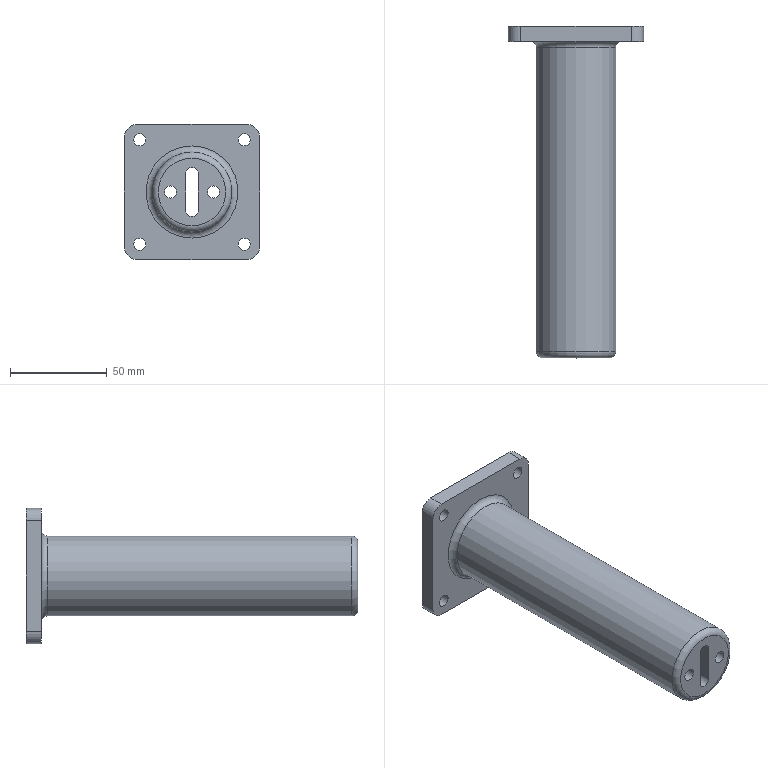Part | NX | features MG0330 trunion parts 24(stanchion group) 2 | 1 solid | 32 faces | box 69.85 x 171.45 x 69.85 mm | volume 105994 mm3 | cylinder 15 | plane 11 | torus 4 | cone 2 | commonest cylinder face diameters 6.35 x6 12.7 x4 6.401 x2 34.925 x2 41.275 x1
STEP:
#1=CARTESIAN_POINT('',(0.,285.75,17.971));
#2=VERTEX_POINT('',#1);
#3=CARTESIAN_POINT('',(0.,285.75,0.));
#4=DIRECTION('',(0.,1.,0.));
#5=DIRECTION('',(0.,0.,1.));
#6=AXIS2_PLACEMENT_3D('',#3,#4,#5);
#7=CIRCLE('',#6,17.971);
#8=EDGE_CURVE('',#2,#2,#7,.F.);
#9=ORIENTED_EDGE('',*,*,#8,.T.);
#10=EDGE_LOOP('',(#9));
#11=FACE_BOUND('',#10,.T.);
#12=CARTESIAN_POINT('',(-26.988,285.75,-23.812));
#13=VERTEX_POINT('',#12);
#14=CARTESIAN_POINT('',(-26.988,285.75,-26.988));
#15=DIRECTION('',(0.,1.,0.));
#16=DIRECTION('',(0.,0.,1.));
#17=AXIS2_PLACEMENT_3D('',#14,#15,#16);
#18=CIRCLE('',#17,3.175);
#19=EDGE_CURVE('',#13,#13,#18,.T.);
#20=ORIENTED_EDGE('',*,*,#19,.F.);
#21=EDGE_LOOP('',(#20));
#22=FACE_BOUND('',#21,.T.);
#23=CARTESIAN_POINT('',(26.988,285.75,-23.812));
#24=VERTEX_POINT('',#23);
#25=CARTESIAN_POINT('',(26.988,285.75,-26.988));
#26=DIRECTION('',(0.,1.,0.));
#27=DIRECTION('',(0.,0.,1.));
#28=AXIS2_PLACEMENT_3D('',#25,#26,#27);
#29=CIRCLE('',#28,3.175);
#30=EDGE_CURVE('',#24,#24,#29,.T.);
#31=ORIENTED_EDGE('',*,*,#30,.F.);
#32=EDGE_LOOP('',(#31));
#33=FACE_BOUND('',#32,.T.);
#34=CARTESIAN_POINT('',(26.988,285.75,30.163));
#35=VERTEX_POINT('',#34);
#36=CARTESIAN_POINT('',(26.988,285.75,26.988));
#37=DIRECTION('',(0.,1.,0.));
#38=DIRECTION('',(0.,0.,1.));
#39=AXIS2_PLACEMENT_3D('',#36,#37,#38);
#40=CIRCLE('',#39,3.175);
#41=EDGE_CURVE('',#35,#35,#40,.T.);
#42=ORIENTED_EDGE('',*,*,#41,.F.);
#43=EDGE_LOOP('',(#42));
#44=FACE_BOUND('',#43,.T.);
#45=CARTESIAN_POINT('',(-26.988,285.75,30.163));
#46=VERTEX_POINT('',#45);
#47=CARTESIAN_POINT('',(-26.988,285.75,26.988));
#48=DIRECTION('',(0.,1.,0.));
#49=DIRECTION('',(0.,0.,1.));
#50=AXIS2_PLACEMENT_3D('',#47,#48,#49);
#51=CIRCLE('',#50,3.175);
#52=EDGE_CURVE('',#46,#46,#51,.T.);
#53=ORIENTED_EDGE('',*,*,#52,.F.);
#54=EDGE_LOOP('',(#53));
#55=FACE_BOUND('',#54,.T.);
#56=CARTESIAN_POINT('',(28.575,285.75,-34.925));
#57=VERTEX_POINT('',#56);
#58=CARTESIAN_POINT('',(-28.575,285.75,-34.925));
#59=VERTEX_POINT('',#58);
#60=CARTESIAN_POINT('',(34.925,285.75,-34.925));
#61=DIRECTION('',(-1.,0.,0.));
#62=VECTOR('',#61,1000.);
#63=LINE('',#60,#62);
#64=EDGE_CURVE('',#57,#59,#63,.T.);
#65=ORIENTED_EDGE('',*,*,#64,.T.);
#66=CARTESIAN_POINT('',(-34.925,285.75,-28.575));
#67=VERTEX_POINT('',#66);
#68=CARTESIAN_POINT('',(-28.575,285.75,-28.575));
#69=DIRECTION('',(0.,1.,0.));
#70=DIRECTION('',(0.,0.,1.));
#71=AXIS2_PLACEMENT_3D('',#68,#69,#70);
#72=CIRCLE('',#71,6.35);
#73=EDGE_CURVE('',#59,#67,#72,.T.);
#74=ORIENTED_EDGE('',*,*,#73,.T.);
#75=CARTESIAN_POINT('',(-34.925,285.75,28.575));
#76=VERTEX_POINT('',#75);
#77=CARTESIAN_POINT('',(-34.925,285.75,-34.925));
#78=DIRECTION('',(0.,0.,1.));
#79=VECTOR('',#78,1000.);
#80=LINE('',#77,#79);
#81=EDGE_CURVE('',#67,#76,#80,.T.);
#82=ORIENTED_EDGE('',*,*,#81,.T.);
#83=CARTESIAN_POINT('',(-28.575,285.75,34.925));
#84=VERTEX_POINT('',#83);
#85=CARTESIAN_POINT('',(-28.575,285.75,28.575));
#86=DIRECTION('',(0.,1.,0.));
#87=DIRECTION('',(0.,0.,1.));
#88=AXIS2_PLACEMENT_3D('',#85,#86,#87);
#89=CIRCLE('',#88,6.35);
#90=EDGE_CURVE('',#76,#84,#89,.T.);
#91=ORIENTED_EDGE('',*,*,#90,.T.);
#92=CARTESIAN_POINT('',(28.575,285.75,34.925));
#93=VERTEX_POINT('',#92);
#94=CARTESIAN_POINT('',(34.925,285.75,34.925));
#95=DIRECTION('',(1.,0.,0.));
#96=VECTOR('',#95,1000.);
#97=LINE('',#94,#96);
#98=EDGE_CURVE('',#84,#93,#97,.T.);
#99=ORIENTED_EDGE('',*,*,#98,.T.);
#100=CARTESIAN_POINT('',(34.925,285.75,28.575));
#101=VERTEX_POINT('',#100);
#102=CARTESIAN_POINT('',(28.575,285.75,28.575));
#103=DIRECTION('',(0.,1.,0.));
#104=DIRECTION('',(0.,0.,1.));
#105=AXIS2_PLACEMENT_3D('',#102,#103,#104);
#106=CIRCLE('',#105,6.35);
#107=EDGE_CURVE('',#93,#101,#106,.T.);
#108=ORIENTED_EDGE('',*,*,#107,.T.);
#109=CARTESIAN_POINT('',(34.925,285.75,-28.575));
#110=VERTEX_POINT('',#109);
#111=CARTESIAN_POINT('',(34.925,285.75,-34.925));
#112=DIRECTION('',(0.,0.,-1.));
#113=VECTOR('',#112,1000.);
#114=LINE('',#111,#113);
#115=EDGE_CURVE('',#101,#110,#114,.T.);
#116=ORIENTED_EDGE('',*,*,#115,.T.);
#117=CARTESIAN_POINT('',(28.575,285.75,-28.575));
#118=DIRECTION('',(0.,1.,0.));
#119=DIRECTION('',(0.,0.,1.));
#120=AXIS2_PLACEMENT_3D('',#117,#118,#119);
#121=CIRCLE('',#120,6.35);
#122=EDGE_CURVE('',#110,#57,#121,.T.);
#123=ORIENTED_EDGE('',*,*,#122,.T.);
#124=EDGE_LOOP('',(#65,#74,#82,#91,#99,#108,#116,#123));
#125=FACE_BOUND('',#124,.T.);
#126=CARTESIAN_POINT('',(17.462,285.75,0.));
#127=DIRECTION('',(0.,1.,0.));
#128=DIRECTION('',(0.,0.,1.));
#129=AXIS2_PLACEMENT_3D('',#126,#127,#128);
#130=PLANE('',#129);
#131=ADVANCED_FACE('',(#11,#22,#33,#44,#55,#125),#130,.T.);
#132=CARTESIAN_POINT('',(0.,285.242,17.462));
#133=VERTEX_POINT('',#132);
#134=CARTESIAN_POINT('',(0.,285.242,0.));
#135=DIRECTION('',(0.,1.,0.));
#136=DIRECTION('',(0.,0.,1.));
#137=AXIS2_PLACEMENT_3D('',#134,#135,#136);
#138=CIRCLE('',#137,17.462);
#139=EDGE_CURVE('',#133,#133,#138,.T.);
#140=ORIENTED_EDGE('',*,*,#139,.T.);
#141=EDGE_LOOP('',(#140));
#142=FACE_BOUND('',#141,.T.);
#143=CARTESIAN_POINT('',(0.,282.734,-17.462));
#144=VERTEX_POINT('',#143);
#145=CARTESIAN_POINT('',(0.,282.734,0.));
#146=DIRECTION('',(0.,-1.,0.));
#147=DIRECTION('',(0.,0.,-1.));
#148=AXIS2_PLACEMENT_3D('',#145,#146,#147);
#149=CIRCLE('',#148,17.462);
#150=EDGE_CURVE('',#144,#144,#149,.T.);
#151=ORIENTED_EDGE('',*,*,#150,.T.);
#152=EDGE_LOOP('',(#151));
#153=FACE_BOUND('',#152,.T.);
#154=CARTESIAN_POINT('',(0.,0.,0.));
#155=DIRECTION('',(0.,-1.,0.));
#156=DIRECTION('',(0.,0.,-1.));
#157=AXIS2_PLACEMENT_3D('',#154,#155,#156);
#158=CYLINDRICAL_SURFACE('',#157,17.462);
#159=ADVANCED_FACE('',(#142,#153),#158,.F.);
#160=CARTESIAN_POINT('',(0.,282.734,-17.64));
#161=VERTEX_POINT('',#160);
#162=CARTESIAN_POINT('',(0.,282.734,0.));
#163=DIRECTION('',(0.,-1.,0.));
#164=DIRECTION('',(0.,0.,-1.));
#165=AXIS2_PLACEMENT_3D('',#162,#163,#164);
#166=CIRCLE('',#165,17.64);
#167=EDGE_CURVE('',#161,#161,#166,.T.);
#168=ORIENTED_EDGE('',*,*,#167,.T.);
#169=EDGE_LOOP('',(#168));
#170=FACE_BOUND('',#169,.T.);
#171=ORIENTED_EDGE('',*,*,#150,.F.);
#172=EDGE_LOOP('',(#171));
#173=FACE_BOUND('',#172,.T.);
#174=CARTESIAN_POINT('',(17.64,282.734,0.));
#175=DIRECTION('',(0.,-1.,0.));
#176=DIRECTION('',(0.,0.,-1.));
#177=AXIS2_PLACEMENT_3D('',#174,#175,#176);
#178=PLANE('',#177);
#179=ADVANCED_FACE('',(#170,#173),#178,.T.);
#180=CARTESIAN_POINT('',(0.,281.379,-18.202));
#181=VERTEX_POINT('',#180);
#182=CARTESIAN_POINT('',(0.,281.379,0.));
#183=DIRECTION('',(0.,-1.,0.));
#184=DIRECTION('',(0.,0.,-1.));
#185=AXIS2_PLACEMENT_3D('',#182,#183,#184);
#186=CIRCLE('',#185,18.202);
#187=EDGE_CURVE('',#181,#181,#186,.T.);
#188=ORIENTED_EDGE('',*,*,#187,.T.);
#189=EDGE_LOOP('',(#188));
#190=FACE_BOUND('',#189,.T.);
#191=ORIENTED_EDGE('',*,*,#167,.F.);
#192=EDGE_LOOP('',(#191));
#193=FACE_BOUND('',#192,.T.);
#194=CARTESIAN_POINT('',(0.,281.94,0.));
#195=DIRECTION('',(0.,-1.,0.));
#196=DIRECTION('',(0.,0.,-1.));
#197=AXIS2_PLACEMENT_3D('',#194,#195,#196);
#198=TOROIDAL_SURFACE('',#197,17.64,0.7937);
#199=ADVANCED_FACE('',(#190,#193),#198,.F.);
#200=CARTESIAN_POINT('',(0.,280.64,-17.462));
#201=VERTEX_POINT('',#200);
#202=CARTESIAN_POINT('',(0.,280.64,0.));
#203=DIRECTION('',(0.,-1.,0.));
#204=DIRECTION('',(0.,0.,-1.));
#205=AXIS2_PLACEMENT_3D('',#202,#203,#204);
#206=CIRCLE('',#205,17.462);
#207=EDGE_CURVE('',#201,#201,#206,.T.);
#208=ORIENTED_EDGE('',*,*,#207,.T.);
#209=EDGE_LOOP('',(#208));
#210=FACE_BOUND('',#209,.T.);
#211=ORIENTED_EDGE('',*,*,#187,.F.);
#212=EDGE_LOOP('',(#211));
#213=FACE_BOUND('',#212,.T.);
#214=CARTESIAN_POINT('',(0.,281.379,0.));
#215=DIRECTION('',(0.,1.,0.));
#216=DIRECTION('',(0.,0.,1.));
#217=AXIS2_PLACEMENT_3D('',#214,#215,#216);
#218=CONICAL_SURFACE('',#217,18.202,0.7854);
#219=ADVANCED_FACE('',(#210,#213),#218,.F.);
#220=CARTESIAN_POINT('',(0.,134.925,-17.462));
#221=VERTEX_POINT('',#220);
#222=CARTESIAN_POINT('',(0.,134.925,0.));
#223=DIRECTION('',(0.,-1.,0.));
#224=DIRECTION('',(0.,0.,-1.));
#225=AXIS2_PLACEMENT_3D('',#222,#223,#224);
#226=CIRCLE('',#225,17.462);
#227=EDGE_CURVE('',#221,#221,#226,.T.);
#228=ORIENTED_EDGE('',*,*,#227,.T.);
#229=EDGE_LOOP('',(#228));
#230=FACE_BOUND('',#229,.T.);
#231=ORIENTED_EDGE('',*,*,#207,.F.);
#232=EDGE_LOOP('',(#231));
#233=FACE_BOUND('',#232,.T.);
#234=CARTESIAN_POINT('',(0.,0.,0.));
#235=DIRECTION('',(0.,-1.,0.));
#236=DIRECTION('',(0.,0.,-1.));
#237=AXIS2_PLACEMENT_3D('',#234,#235,#236);
#238=CYLINDRICAL_SURFACE('',#237,17.462);
#239=ADVANCED_FACE('',(#230,#233),#238,.F.);
#240=CARTESIAN_POINT('',(0.,133.35,-15.888));
#241=VERTEX_POINT('',#240);
#242=CARTESIAN_POINT('',(0.,133.35,0.));
#243=DIRECTION('',(0.,-1.,0.));
#244=DIRECTION('',(0.,0.,-1.));
#245=AXIS2_PLACEMENT_3D('',#242,#243,#244);
#246=CIRCLE('',#245,15.888);
#247=EDGE_CURVE('',#241,#241,#246,.T.);
#248=ORIENTED_EDGE('',*,*,#247,.T.);
#249=EDGE_LOOP('',(#248));
#250=FACE_BOUND('',#249,.T.);
#251=ORIENTED_EDGE('',*,*,#227,.F.);
#252=EDGE_LOOP('',(#251));
#253=FACE_BOUND('',#252,.T.);
#254=CARTESIAN_POINT('',(0.,134.925,0.));
#255=DIRECTION('',(0.,-1.,0.));
#256=DIRECTION('',(0.,0.,-1.));
#257=AXIS2_PLACEMENT_3D('',#254,#255,#256);
#258=TOROIDAL_SURFACE('',#257,15.888,1.575);
#259=ADVANCED_FACE('',(#250,#253),#258,.F.);
#260=CARTESIAN_POINT('',(-11.113,133.35,-3.175));
#261=VERTEX_POINT('',#260);
#262=CARTESIAN_POINT('',(-11.113,133.35,0.));
#263=DIRECTION('',(0.,-1.,0.));
#264=DIRECTION('',(0.,0.,-1.));
#265=AXIS2_PLACEMENT_3D('',#262,#263,#264);
#266=CIRCLE('',#265,3.175);
#267=EDGE_CURVE('',#261,#261,#266,.T.);
#268=ORIENTED_EDGE('',*,*,#267,.T.);
#269=EDGE_LOOP('',(#268));
#270=FACE_BOUND('',#269,.T.);
#271=CARTESIAN_POINT('',(11.113,133.35,-3.175));
#272=VERTEX_POINT('',#271);
#273=CARTESIAN_POINT('',(11.113,133.35,0.));
#274=DIRECTION('',(0.,-1.,0.));
#275=DIRECTION('',(0.,0.,-1.));
#276=AXIS2_PLACEMENT_3D('',#273,#274,#275);
#277=CIRCLE('',#276,3.175);
#278=EDGE_CURVE('',#272,#272,#277,.T.);
#279=ORIENTED_EDGE('',*,*,#278,.T.);
#280=EDGE_LOOP('',(#279));
#281=FACE_BOUND('',#280,.T.);
#282=CARTESIAN_POINT('',(-3.2,133.35,-9.525));
#283=VERTEX_POINT('',#282);
#284=CARTESIAN_POINT('',(3.2,133.35,-9.525));
#285=VERTEX_POINT('',#284);
#286=CARTESIAN_POINT('',(0.,133.35,-9.525));
#287=DIRECTION('',(0.,-1.,0.));
#288=DIRECTION('',(0.,0.,-1.));
#289=AXIS2_PLACEMENT_3D('',#286,#287,#288);
#290=CIRCLE('',#289,3.2);
#291=EDGE_CURVE('',#283,#285,#290,.T.);
#292=ORIENTED_EDGE('',*,*,#291,.T.);
#293=CARTESIAN_POINT('',(3.2,133.35,9.525));
#294=VERTEX_POINT('',#293);
#295=CARTESIAN_POINT('',(3.2,133.35,-9.525));
#296=DIRECTION('',(0.,0.,1.));
#297=VECTOR('',#296,1000.);
#298=LINE('',#295,#297);
#299=EDGE_CURVE('',#285,#294,#298,.T.);
#300=ORIENTED_EDGE('',*,*,#299,.T.);
#301=CARTESIAN_POINT('',(-3.2,133.35,9.525));
#302=VERTEX_POINT('',#301);
#303=CARTESIAN_POINT('',(0.,133.35,9.525));
#304=DIRECTION('',(0.,-1.,0.));
#305=DIRECTION('',(0.,0.,-1.));
#306=AXIS2_PLACEMENT_3D('',#303,#304,#305);
#307=CIRCLE('',#306,3.2);
#308=EDGE_CURVE('',#294,#302,#307,.T.);
#309=ORIENTED_EDGE('',*,*,#308,.T.);
#310=CARTESIAN_POINT('',(-3.2,133.35,-9.525));
#311=DIRECTION('',(0.,0.,-1.));
#312=VECTOR('',#311,1000.);
#313=LINE('',#310,#312);
#314=EDGE_CURVE('',#302,#283,#313,.T.);
#315=ORIENTED_EDGE('',*,*,#314,.T.);
#316=EDGE_LOOP('',(#292,#300,#309,#315));
#317=FACE_BOUND('',#316,.T.);
#318=ORIENTED_EDGE('',*,*,#247,.F.);
#319=EDGE_LOOP('',(#318));
#320=FACE_BOUND('',#319,.T.);
#321=CARTESIAN_POINT('',(15.888,133.35,0.));
#322=DIRECTION('',(0.,1.,0.));
#323=DIRECTION('',(0.,0.,1.));
#324=AXIS2_PLACEMENT_3D('',#321,#322,#323);
#325=PLANE('',#324);
#326=ADVANCED_FACE('',(#270,#281,#317,#320),#325,.T.);
#327=CARTESIAN_POINT('',(34.925,277.812,28.575));
#328=VERTEX_POINT('',#327);
#329=CARTESIAN_POINT('',(34.925,277.812,-28.575));
#330=VERTEX_POINT('',#329);
#331=CARTESIAN_POINT('',(34.925,277.812,-34.925));
#332=DIRECTION('',(0.,0.,-1.));
#333=VECTOR('',#332,1000.);
#334=LINE('',#331,#333);
#335=EDGE_CURVE('',#328,#330,#334,.T.);
#336=ORIENTED_EDGE('',*,*,#335,.T.);
#337=CARTESIAN_POINT('',(34.925,179.03,-28.575));
#338=DIRECTION('',(0.,1.,0.));
#339=VECTOR('',#338,1000.);
#340=LINE('',#337,#339);
#341=EDGE_CURVE('',#330,#110,#340,.T.);
#342=ORIENTED_EDGE('',*,*,#341,.T.);
#343=ORIENTED_EDGE('',*,*,#115,.F.);
#344=CARTESIAN_POINT('',(34.925,179.03,28.575));
#345=DIRECTION('',(0.,1.,0.));
#346=VECTOR('',#345,1000.);
#347=LINE('',#344,#346);
#348=EDGE_CURVE('',#101,#328,#347,.F.);
#349=ORIENTED_EDGE('',*,*,#348,.T.);
#350=EDGE_LOOP('',(#336,#342,#343,#349));
#351=FACE_BOUND('',#350,.T.);
#352=CARTESIAN_POINT('',(34.925,179.03,-34.925));
#353=DIRECTION('',(1.,0.,0.));
#354=DIRECTION('',(0.,0.,-1.));
#355=AXIS2_PLACEMENT_3D('',#352,#353,#354);
#356=PLANE('',#355);
#357=ADVANCED_FACE('',(#351),#356,.T.);
#358=CARTESIAN_POINT('',(-28.575,277.812,34.925));
#359=VERTEX_POINT('',#358);
#360=CARTESIAN_POINT('',(28.575,277.812,34.925));
#361=VERTEX_POINT('',#360);
#362=CARTESIAN_POINT('',(34.925,277.812,34.925));
#363=DIRECTION('',(1.,0.,0.));
#364=VECTOR('',#363,1000.);
#365=LINE('',#362,#364);
#366=EDGE_CURVE('',#359,#361,#365,.T.);
#367=ORIENTED_EDGE('',*,*,#366,.T.);
#368=CARTESIAN_POINT('',(28.575,179.03,34.925));
#369=DIRECTION('',(0.,1.,0.));
#370=VECTOR('',#369,1000.);
#371=LINE('',#368,#370);
#372=EDGE_CURVE('',#361,#93,#371,.T.);
#373=ORIENTED_EDGE('',*,*,#372,.T.);
#374=ORIENTED_EDGE('',*,*,#98,.F.);
#375=CARTESIAN_POINT('',(-28.575,179.03,34.925));
#376=DIRECTION('',(0.,1.,0.));
#377=VECTOR('',#376,1000.);
#378=LINE('',#375,#377);
#379=EDGE_CURVE('',#84,#359,#378,.F.);
#380=ORIENTED_EDGE('',*,*,#379,.T.);
#381=EDGE_LOOP('',(#367,#373,#374,#380));
#382=FACE_BOUND('',#381,.T.);
#383=CARTESIAN_POINT('',(34.925,179.03,34.925));
#384=DIRECTION('',(0.,0.,1.));
#385=DIRECTION('',(1.,0.,0.));
#386=AXIS2_PLACEMENT_3D('',#383,#384,#385);
#387=PLANE('',#386);
#388=ADVANCED_FACE('',(#382),#387,.T.);
#389=ORIENTED_EDGE('',*,*,#81,.F.);
#390=CARTESIAN_POINT('',(-34.925,277.812,-28.575));
#391=VERTEX_POINT('',#390);
#392=CARTESIAN_POINT('',(-34.925,179.03,-28.575));
#393=DIRECTION('',(0.,1.,0.));
#394=VECTOR('',#393,1000.);
#395=LINE('',#392,#394);
#396=EDGE_CURVE('',#67,#391,#395,.F.);
#397=ORIENTED_EDGE('',*,*,#396,.T.);
#398=CARTESIAN_POINT('',(-34.925,277.812,28.575));
#399=VERTEX_POINT('',#398);
#400=CARTESIAN_POINT('',(-34.925,277.812,-34.925));
#401=DIRECTION('',(0.,0.,1.));
#402=VECTOR('',#401,1000.);
#403=LINE('',#400,#402);
#404=EDGE_CURVE('',#391,#399,#403,.T.);
#405=ORIENTED_EDGE('',*,*,#404,.T.);
#406=CARTESIAN_POINT('',(-34.925,179.03,28.575));
#407=DIRECTION('',(0.,1.,0.));
#408=VECTOR('',#407,1000.);
#409=LINE('',#406,#408);
#410=EDGE_CURVE('',#399,#76,#409,.T.);
#411=ORIENTED_EDGE('',*,*,#410,.T.);
#412=EDGE_LOOP('',(#389,#397,#405,#411));
#413=FACE_BOUND('',#412,.T.);
#414=CARTESIAN_POINT('',(-34.925,179.03,-34.925));
#415=DIRECTION('',(-1.,0.,0.));
#416=DIRECTION('',(0.,0.,1.));
#417=AXIS2_PLACEMENT_3D('',#414,#415,#416);
#418=PLANE('',#417);
#419=ADVANCED_FACE('',(#413),#418,.T.);
#420=CARTESIAN_POINT('',(28.575,277.812,-34.925));
#421=VERTEX_POINT('',#420);
#422=CARTESIAN_POINT('',(-28.575,277.812,-34.925));
#423=VERTEX_POINT('',#422);
#424=CARTESIAN_POINT('',(34.925,277.812,-34.925));
#425=DIRECTION('',(-1.,0.,0.));
#426=VECTOR('',#425,1000.);
#427=LINE('',#424,#426);
#428=EDGE_CURVE('',#421,#423,#427,.T.);
#429=ORIENTED_EDGE('',*,*,#428,.T.);
#430=CARTESIAN_POINT('',(-28.575,179.03,-34.925));
#431=DIRECTION('',(0.,1.,0.));
#432=VECTOR('',#431,1000.);
#433=LINE('',#430,#432);
#434=EDGE_CURVE('',#423,#59,#433,.T.);
#435=ORIENTED_EDGE('',*,*,#434,.T.);
#436=ORIENTED_EDGE('',*,*,#64,.F.);
#437=CARTESIAN_POINT('',(28.575,179.03,-34.925));
#438=DIRECTION('',(0.,1.,0.));
#439=VECTOR('',#438,1000.);
#440=LINE('',#437,#439);
#441=EDGE_CURVE('',#57,#421,#440,.F.);
#442=ORIENTED_EDGE('',*,*,#441,.T.);
#443=EDGE_LOOP('',(#429,#435,#436,#442));
#444=FACE_BOUND('',#443,.T.);
#445=CARTESIAN_POINT('',(34.925,179.03,-34.925));
#446=DIRECTION('',(0.,0.,-1.));
#447=DIRECTION('',(-1.,0.,0.));
#448=AXIS2_PLACEMENT_3D('',#445,#446,#447);
#449=PLANE('',#448);
#450=ADVANCED_FACE('',(#444),#449,.T.);
#451=ORIENTED_EDGE('',*,*,#52,.T.);
#452=EDGE_LOOP('',(#451));
#453=FACE_BOUND('',#452,.T.);
#454=CARTESIAN_POINT('',(-26.988,277.812,23.812));
#455=VERTEX_POINT('',#454);
#456=CARTESIAN_POINT('',(-26.988,277.812,26.988));
#457=DIRECTION('',(0.,-1.,0.));
#458=DIRECTION('',(0.,0.,-1.));
#459=AXIS2_PLACEMENT_3D('',#456,#457,#458);
#460=CIRCLE('',#459,3.175);
#461=EDGE_CURVE('',#455,#455,#460,.F.);
#462=ORIENTED_EDGE('',*,*,#461,.F.);
#463=EDGE_LOOP('',(#462));
#464=FACE_BOUND('',#463,.T.);
#465=CARTESIAN_POINT('',(-26.988,179.03,26.988));
#466=DIRECTION('',(0.,1.,0.));
#467=DIRECTION('',(0.,0.,1.));
#468=AXIS2_PLACEMENT_3D('',#465,#466,#467);
#469=CYLINDRICAL_SURFACE('',#468,3.175);
#470=ADVANCED_FACE('',(#453,#464),#469,.F.);
#471=ORIENTED_EDGE('',*,*,#41,.T.);
#472=EDGE_LOOP('',(#471));
#473=FACE_BOUND('',#472,.T.);
#474=CARTESIAN_POINT('',(26.988,277.812,23.812));
#475=VERTEX_POINT('',#474);
#476=CARTESIAN_POINT('',(26.988,277.812,26.988));
#477=DIRECTION('',(0.,-1.,0.));
#478=DIRECTION('',(0.,0.,-1.));
#479=AXIS2_PLACEMENT_3D('',#476,#477,#478);
#480=CIRCLE('',#479,3.175);
#481=EDGE_CURVE('',#475,#475,#480,.F.);
#482=ORIENTED_EDGE('',*,*,#481,.F.);
#483=EDGE_LOOP('',(#482));
#484=FACE_BOUND('',#483,.T.);
#485=CARTESIAN_POINT('',(26.988,179.03,26.988));
#486=DIRECTION('',(0.,1.,0.));
#487=DIRECTION('',(0.,0.,1.));
#488=AXIS2_PLACEMENT_3D('',#485,#486,#487);
#489=CYLINDRICAL_SURFACE('',#488,3.175);
#490=ADVANCED_FACE('',(#473,#484),#489,.F.);
#491=ORIENTED_EDGE('',*,*,#30,.T.);
#492=EDGE_LOOP('',(#491));
#493=FACE_BOUND('',#492,.T.);
#494=CARTESIAN_POINT('',(26.988,277.812,-30.163));
#495=VERTEX_POINT('',#494);
#496=CARTESIAN_POINT('',(26.988,277.812,-26.988));
#497=DIRECTION('',(0.,-1.,0.));
#498=DIRECTION('',(0.,0.,-1.));
#499=AXIS2_PLACEMENT_3D('',#496,#497,#498);
#500=CIRCLE('',#499,3.175);
#501=EDGE_CURVE('',#495,#495,#500,.F.);
#502=ORIENTED_EDGE('',*,*,#501,.F.);
#503=EDGE_LOOP('',(#502));
#504=FACE_BOUND('',#503,.T.);
#505=CARTESIAN_POINT('',(26.988,179.03,-26.988));
#506=DIRECTION('',(0.,1.,0.));
#507=DIRECTION('',(0.,0.,1.));
#508=AXIS2_PLACEMENT_3D('',#505,#506,#507);
#509=CYLINDRICAL_SURFACE('',#508,3.175);
#510=ADVANCED_FACE('',(#493,#504),#509,.F.);
#511=ORIENTED_EDGE('',*,*,#19,.T.);
#512=EDGE_LOOP('',(#511));
#513=FACE_BOUND('',#512,.T.);
#514=CARTESIAN_POINT('',(-26.988,277.812,-30.163));
#515=VERTEX_POINT('',#514);
#516=CARTESIAN_POINT('',(-26.988,277.812,-26.988));
#517=DIRECTION('',(0.,-1.,0.));
#518=DIRECTION('',(0.,0.,-1.));
#519=AXIS2_PLACEMENT_3D('',#516,#517,#518);
#520=CIRCLE('',#519,3.175);
#521=EDGE_CURVE('',#515,#515,#520,.F.);
#522=ORIENTED_EDGE('',*,*,#521,.F.);
#523=EDGE_LOOP('',(#522));
#524=FACE_BOUND('',#523,.T.);
#525=CARTESIAN_POINT('',(-26.988,179.03,-26.988));
#526=DIRECTION('',(0.,1.,0.));
#527=DIRECTION('',(0.,0.,1.));
#528=AXIS2_PLACEMENT_3D('',#525,#526,#527);
#529=CYLINDRICAL_SURFACE('',#528,3.175);
#530=ADVANCED_FACE('',(#513,#524),#529,.F.);
#531=CARTESIAN_POINT('',(-11.113,114.3,-3.175));
#532=VERTEX_POINT('',#531);
#533=CARTESIAN_POINT('',(-11.113,114.3,0.));
#534=DIRECTION('',(0.,-1.,0.));
#535=DIRECTION('',(0.,0.,-1.));
#536=AXIS2_PLACEMENT_3D('',#533,#534,#535);
#537=CIRCLE('',#536,3.175);
#538=EDGE_CURVE('',#532,#532,#537,.T.);
#539=ORIENTED_EDGE('',*,*,#538,.F.);
#540=EDGE_LOOP('',(#539));
#541=FACE_BOUND('',#540,.T.);
#542=CARTESIAN_POINT('',(11.113,114.3,-3.175));
#543=VERTEX_POINT('',#542);
#544=CARTESIAN_POINT('',(11.113,114.3,0.));
#545=DIRECTION('',(0.,-1.,0.));
#546=DIRECTION('',(0.,0.,-1.));
#547=AXIS2_PLACEMENT_3D('',#544,#545,#546);
#548=CIRCLE('',#547,3.175);
#549=EDGE_CURVE('',#543,#543,#548,.T.);
#550=ORIENTED_EDGE('',*,*,#549,.F.);
#551=EDGE_LOOP('',(#550));
#552=FACE_BOUND('',#551,.T.);
#553=CARTESIAN_POINT('',(-3.2,114.3,-9.525));
#554=VERTEX_POINT('',#553);
#555=CARTESIAN_POINT('',(3.2,114.3,-9.525));
#556=VERTEX_POINT('',#555);
#557=CARTESIAN_POINT('',(0.,114.3,-9.525));
#558=DIRECTION('',(0.,-1.,0.));
#559=DIRECTION('',(0.,0.,-1.));
#560=AXIS2_PLACEMENT_3D('',#557,#558,#559);
#561=CIRCLE('',#560,3.2);
#562=EDGE_CURVE('',#554,#556,#561,.T.);
#563=ORIENTED_EDGE('',*,*,#562,.F.);
#564=CARTESIAN_POINT('',(-3.2,114.3,9.525));
#565=VERTEX_POINT('',#564);
#566=CARTESIAN_POINT('',(-3.2,114.3,-9.525));
#567=DIRECTION('',(0.,0.,-1.));
#568=VECTOR('',#567,1000.);
#569=LINE('',#566,#568);
#570=EDGE_CURVE('',#565,#554,#569,.T.);
#571=ORIENTED_EDGE('',*,*,#570,.F.);
#572=CARTESIAN_POINT('',(3.2,114.3,9.525));
#573=VERTEX_POINT('',#572);
#574=CARTESIAN_POINT('',(0.,114.3,9.525));
#575=DIRECTION('',(0.,-1.,0.));
#576=DIRECTION('',(0.,0.,-1.));
#577=AXIS2_PLACEMENT_3D('',#574,#575,#576);
#578=CIRCLE('',#577,3.2);
#579=EDGE_CURVE('',#573,#565,#578,.T.);
#580=ORIENTED_EDGE('',*,*,#579,.F.);
#581=CARTESIAN_POINT('',(3.2,114.3,-9.525));
#582=DIRECTION('',(0.,0.,1.));
#583=VECTOR('',#582,1000.);
#584=LINE('',#581,#583);
#585=EDGE_CURVE('',#556,#573,#584,.T.);
#586=ORIENTED_EDGE('',*,*,#585,.F.);
#587=EDGE_LOOP('',(#563,#571,#580,#586));
#588=FACE_BOUND('',#587,.T.);
#589=CARTESIAN_POINT('',(0.,114.3,-17.462));
#590=VERTEX_POINT('',#589);
#591=CARTESIAN_POINT('',(0.,114.3,0.));
#592=DIRECTION('',(0.,-1.,0.));
#593=DIRECTION('',(0.,0.,-1.));
#594=AXIS2_PLACEMENT_3D('',#591,#592,#593);
#595=CIRCLE('',#594,17.462);
#596=EDGE_CURVE('',#590,#590,#595,.T.);
#597=ORIENTED_EDGE('',*,*,#596,.T.);
#598=EDGE_LOOP('',(#597));
#599=FACE_BOUND('',#598,.T.);
#600=CARTESIAN_POINT('',(17.462,114.3,0.));
#601=DIRECTION('',(0.,-1.,0.));
#602=DIRECTION('',(0.,0.,-1.));
#603=AXIS2_PLACEMENT_3D('',#600,#601,#602);
#604=PLANE('',#603);
#605=ADVANCED_FACE('',(#541,#552,#588,#599),#604,.T.);
#606=CARTESIAN_POINT('',(0.,117.475,-20.637));
#607=VERTEX_POINT('',#606);
#608=CARTESIAN_POINT('',(0.,117.475,0.));
#609=DIRECTION('',(0.,-1.,0.));
#610=DIRECTION('',(0.,0.,-1.));
#611=AXIS2_PLACEMENT_3D('',#608,#609,#610);
#612=CIRCLE('',#611,20.637);
#613=EDGE_CURVE('',#607,#607,#612,.T.);
#614=ORIENTED_EDGE('',*,*,#613,.T.);
#615=EDGE_LOOP('',(#614));
#616=FACE_BOUND('',#615,.T.);
#617=ORIENTED_EDGE('',*,*,#596,.F.);
#618=EDGE_LOOP('',(#617));
#619=FACE_BOUND('',#618,.T.);
#620=CARTESIAN_POINT('',(0.,117.475,0.));
#621=DIRECTION('',(0.,-1.,0.));
#622=DIRECTION('',(0.,0.,-1.));
#623=AXIS2_PLACEMENT_3D('',#620,#621,#622);
#624=TOROIDAL_SURFACE('',#623,17.462,3.175);
#625=ADVANCED_FACE('',(#616,#619),#624,.T.);
#626=CARTESIAN_POINT('',(0.,274.637,-20.637));
#627=VERTEX_POINT('',#626);
#628=CARTESIAN_POINT('',(0.,274.637,0.));
#629=DIRECTION('',(0.,-1.,0.));
#630=DIRECTION('',(0.,0.,-1.));
#631=AXIS2_PLACEMENT_3D('',#628,#629,#630);
#632=CIRCLE('',#631,20.637);
#633=EDGE_CURVE('',#627,#627,#632,.T.);
#634=ORIENTED_EDGE('',*,*,#633,.T.);
#635=EDGE_LOOP('',(#634));
#636=FACE_BOUND('',#635,.T.);
#637=ORIENTED_EDGE('',*,*,#613,.F.);
#638=EDGE_LOOP('',(#637));
#639=FACE_BOUND('',#638,.T.);
#640=CARTESIAN_POINT('',(0.,0.,0.));
#641=DIRECTION('',(0.,-1.,0.));
#642=DIRECTION('',(0.,0.,-1.));
#643=AXIS2_PLACEMENT_3D('',#640,#641,#642);
#644=CYLINDRICAL_SURFACE('',#643,20.637);
#645=ADVANCED_FACE('',(#636,#639),#644,.T.);
#646=CARTESIAN_POINT('',(0.,277.812,-23.812));
#647=VERTEX_POINT('',#646);
#648=CARTESIAN_POINT('',(0.,277.812,0.));
#649=DIRECTION('',(0.,-1.,0.));
#650=DIRECTION('',(0.,0.,-1.));
#651=AXIS2_PLACEMENT_3D('',#648,#649,#650);
#652=CIRCLE('',#651,23.812);
#653=EDGE_CURVE('',#647,#647,#652,.F.);
#654=ORIENTED_EDGE('',*,*,#653,.T.);
#655=EDGE_LOOP('',(#654));
#656=FACE_BOUND('',#655,.T.);
#657=ORIENTED_EDGE('',*,*,#404,.F.);
#658=CARTESIAN_POINT('',(-28.575,277.812,-28.575));
#659=DIRECTION('',(0.,-1.,0.));
#660=DIRECTION('',(0.,0.,-1.));
#661=AXIS2_PLACEMENT_3D('',#658,#659,#660);
#662=CIRCLE('',#661,6.35);
#663=EDGE_CURVE('',#391,#423,#662,.T.);
#664=ORIENTED_EDGE('',*,*,#663,.T.);
#665=ORIENTED_EDGE('',*,*,#428,.F.);
#666=CARTESIAN_POINT('',(28.575,277.812,-28.575));
#667=DIRECTION('',(0.,-1.,0.));
#668=DIRECTION('',(0.,0.,-1.));
#669=AXIS2_PLACEMENT_3D('',#666,#667,#668);
#670=CIRCLE('',#669,6.35);
#671=EDGE_CURVE('',#421,#330,#670,.T.);
#672=ORIENTED_EDGE('',*,*,#671,.T.);
#673=ORIENTED_EDGE('',*,*,#335,.F.);
#674=CARTESIAN_POINT('',(28.575,277.812,28.575));
#675=DIRECTION('',(0.,-1.,0.));
#676=DIRECTION('',(0.,0.,-1.));
#677=AXIS2_PLACEMENT_3D('',#674,#675,#676);
#678=CIRCLE('',#677,6.35);
#679=EDGE_CURVE('',#328,#361,#678,.T.);
#680=ORIENTED_EDGE('',*,*,#679,.T.);
#681=ORIENTED_EDGE('',*,*,#366,.F.);
#682=CARTESIAN_POINT('',(-28.575,277.812,28.575));
#683=DIRECTION('',(0.,-1.,0.));
#684=DIRECTION('',(0.,0.,-1.));
#685=AXIS2_PLACEMENT_3D('',#682,#683,#684);
#686=CIRCLE('',#685,6.35);
#687=EDGE_CURVE('',#359,#399,#686,.T.);
#688=ORIENTED_EDGE('',*,*,#687,.T.);
#689=EDGE_LOOP('',(#657,#664,#665,#672,#673,#680,#681,#688));
#690=FACE_BOUND('',#689,.T.);
#691=ORIENTED_EDGE('',*,*,#461,.T.);
#692=EDGE_LOOP('',(#691));
#693=FACE_BOUND('',#692,.T.);
#694=ORIENTED_EDGE('',*,*,#501,.T.);
#695=EDGE_LOOP('',(#694));
#696=FACE_BOUND('',#695,.T.);
#697=ORIENTED_EDGE('',*,*,#521,.T.);
#698=EDGE_LOOP('',(#697));
#699=FACE_BOUND('',#698,.T.);
#700=ORIENTED_EDGE('',*,*,#481,.T.);
#701=EDGE_LOOP('',(#700));
#702=FACE_BOUND('',#701,.T.);
#703=CARTESIAN_POINT('',(25.4,277.812,0.));
#704=DIRECTION('',(0.,-1.,0.));
#705=DIRECTION('',(0.,0.,-1.));
#706=AXIS2_PLACEMENT_3D('',#703,#704,#705);
#707=PLANE('',#706);
#708=ADVANCED_FACE('',(#656,#690,#693,#696,#699,#702),#707,.T.);
#709=ORIENTED_EDGE('',*,*,#663,.F.);
#710=ORIENTED_EDGE('',*,*,#396,.F.);
#711=ORIENTED_EDGE('',*,*,#73,.F.);
#712=ORIENTED_EDGE('',*,*,#434,.F.);
#713=EDGE_LOOP('',(#709,#710,#711,#712));
#714=FACE_BOUND('',#713,.T.);
#715=CARTESIAN_POINT('',(-28.575,179.03,-28.575));
#716=DIRECTION('',(0.,1.,0.));
#717=DIRECTION('',(0.,0.,1.));
#718=AXIS2_PLACEMENT_3D('',#715,#716,#717);
#719=CYLINDRICAL_SURFACE('',#718,6.35);
#720=ADVANCED_FACE('',(#714),#719,.T.);
#721=ORIENTED_EDGE('',*,*,#671,.F.);
#722=ORIENTED_EDGE('',*,*,#441,.F.);
#723=ORIENTED_EDGE('',*,*,#122,.F.);
#724=ORIENTED_EDGE('',*,*,#341,.F.);
#725=EDGE_LOOP('',(#721,#722,#723,#724));
#726=FACE_BOUND('',#725,.T.);
#727=CARTESIAN_POINT('',(28.575,179.03,-28.575));
#728=DIRECTION('',(0.,1.,0.));
#729=DIRECTION('',(0.,0.,1.));
#730=AXIS2_PLACEMENT_3D('',#727,#728,#729);
#731=CYLINDRICAL_SURFACE('',#730,6.35);
#732=ADVANCED_FACE('',(#726),#731,.T.);
#733=ORIENTED_EDGE('',*,*,#679,.F.);
#734=ORIENTED_EDGE('',*,*,#348,.F.);
#735=ORIENTED_EDGE('',*,*,#107,.F.);
#736=ORIENTED_EDGE('',*,*,#372,.F.);
#737=EDGE_LOOP('',(#733,#734,#735,#736));
#738=FACE_BOUND('',#737,.T.);
#739=CARTESIAN_POINT('',(28.575,179.03,28.575));
#740=DIRECTION('',(0.,1.,0.));
#741=DIRECTION('',(0.,0.,1.));
#742=AXIS2_PLACEMENT_3D('',#739,#740,#741);
#743=CYLINDRICAL_SURFACE('',#742,6.35);
#744=ADVANCED_FACE('',(#738),#743,.T.);
#745=ORIENTED_EDGE('',*,*,#687,.F.);
#746=ORIENTED_EDGE('',*,*,#379,.F.);
#747=ORIENTED_EDGE('',*,*,#90,.F.);
#748=ORIENTED_EDGE('',*,*,#410,.F.);
#749=EDGE_LOOP('',(#745,#746,#747,#748));
#750=FACE_BOUND('',#749,.T.);
#751=CARTESIAN_POINT('',(-28.575,179.03,28.575));
#752=DIRECTION('',(0.,1.,0.));
#753=DIRECTION('',(0.,0.,1.));
#754=AXIS2_PLACEMENT_3D('',#751,#752,#753);
#755=CYLINDRICAL_SURFACE('',#754,6.35);
#756=ADVANCED_FACE('',(#750),#755,.T.);
#757=ORIENTED_EDGE('',*,*,#562,.T.);
#758=CARTESIAN_POINT('',(3.2,133.35,-9.525));
#759=DIRECTION('',(0.,-1.,0.));
#760=VECTOR('',#759,1000.);
#761=LINE('',#758,#760);
#762=EDGE_CURVE('',#285,#556,#761,.T.);
#763=ORIENTED_EDGE('',*,*,#762,.F.);
#764=ORIENTED_EDGE('',*,*,#291,.F.);
#765=CARTESIAN_POINT('',(-3.2,133.35,-9.525));
#766=DIRECTION('',(0.,-1.,0.));
#767=VECTOR('',#766,1000.);
#768=LINE('',#765,#767);
#769=EDGE_CURVE('',#283,#554,#768,.T.);
#770=ORIENTED_EDGE('',*,*,#769,.T.);
#771=EDGE_LOOP('',(#757,#763,#764,#770));
#772=FACE_BOUND('',#771,.T.);
#773=CARTESIAN_POINT('',(0.,133.35,-9.525));
#774=DIRECTION('',(0.,-1.,0.));
#775=DIRECTION('',(0.,0.,-1.));
#776=AXIS2_PLACEMENT_3D('',#773,#774,#775);
#777=CYLINDRICAL_SURFACE('',#776,3.2);
#778=ADVANCED_FACE('',(#772),#777,.F.);
#779=ORIENTED_EDGE('',*,*,#570,.T.);
#780=ORIENTED_EDGE('',*,*,#769,.F.);
#781=ORIENTED_EDGE('',*,*,#314,.F.);
#782=CARTESIAN_POINT('',(-3.2,133.35,9.525));
#783=DIRECTION('',(0.,-1.,0.));
#784=VECTOR('',#783,1000.);
#785=LINE('',#782,#784);
#786=EDGE_CURVE('',#302,#565,#785,.T.);
#787=ORIENTED_EDGE('',*,*,#786,.T.);
#788=EDGE_LOOP('',(#779,#780,#781,#787));
#789=FACE_BOUND('',#788,.T.);
#790=CARTESIAN_POINT('',(-3.2,133.35,-9.525));
#791=DIRECTION('',(-1.,0.,0.));
#792=DIRECTION('',(0.,0.,1.));
#793=AXIS2_PLACEMENT_3D('',#790,#791,#792);
#794=PLANE('',#793);
#795=ADVANCED_FACE('',(#789),#794,.F.);
#796=ORIENTED_EDGE('',*,*,#579,.T.);
#797=ORIENTED_EDGE('',*,*,#786,.F.);
#798=ORIENTED_EDGE('',*,*,#308,.F.);
#799=CARTESIAN_POINT('',(3.2,133.35,9.525));
#800=DIRECTION('',(0.,-1.,0.));
#801=VECTOR('',#800,1000.);
#802=LINE('',#799,#801);
#803=EDGE_CURVE('',#294,#573,#802,.T.);
#804=ORIENTED_EDGE('',*,*,#803,.T.);
#805=EDGE_LOOP('',(#796,#797,#798,#804));
#806=FACE_BOUND('',#805,.T.);
#807=CARTESIAN_POINT('',(0.,133.35,9.525));
#808=DIRECTION('',(0.,-1.,0.));
#809=DIRECTION('',(0.,0.,-1.));
#810=AXIS2_PLACEMENT_3D('',#807,#808,#809);
#811=CYLINDRICAL_SURFACE('',#810,3.2);
#812=ADVANCED_FACE('',(#806),#811,.F.);
#813=ORIENTED_EDGE('',*,*,#585,.T.);
#814=ORIENTED_EDGE('',*,*,#803,.F.);
#815=ORIENTED_EDGE('',*,*,#299,.F.);
#816=ORIENTED_EDGE('',*,*,#762,.T.);
#817=EDGE_LOOP('',(#813,#814,#815,#816));
#818=FACE_BOUND('',#817,.T.);
#819=CARTESIAN_POINT('',(3.2,133.35,-9.525));
#820=DIRECTION('',(1.,0.,0.));
#821=DIRECTION('',(0.,0.,-1.));
#822=AXIS2_PLACEMENT_3D('',#819,#820,#821);
#823=PLANE('',#822);
#824=ADVANCED_FACE('',(#818),#823,.F.);
#825=ORIENTED_EDGE('',*,*,#278,.F.);
#826=EDGE_LOOP('',(#825));
#827=FACE_BOUND('',#826,.T.);
#828=ORIENTED_EDGE('',*,*,#549,.T.);
#829=EDGE_LOOP('',(#828));
#830=FACE_BOUND('',#829,.T.);
#831=CARTESIAN_POINT('',(11.113,133.35,0.));
#832=DIRECTION('',(0.,-1.,0.));
#833=DIRECTION('',(0.,0.,-1.));
#834=AXIS2_PLACEMENT_3D('',#831,#832,#833);
#835=CYLINDRICAL_SURFACE('',#834,3.175);
#836=ADVANCED_FACE('',(#827,#830),#835,.F.);
#837=ORIENTED_EDGE('',*,*,#267,.F.);
#838=EDGE_LOOP('',(#837));
#839=FACE_BOUND('',#838,.T.);
#840=ORIENTED_EDGE('',*,*,#538,.T.);
#841=EDGE_LOOP('',(#840));
#842=FACE_BOUND('',#841,.T.);
#843=CARTESIAN_POINT('',(-11.113,133.35,0.));
#844=DIRECTION('',(0.,-1.,0.));
#845=DIRECTION('',(0.,0.,-1.));
#846=AXIS2_PLACEMENT_3D('',#843,#844,#845);
#847=CYLINDRICAL_SURFACE('',#846,3.175);
#848=ADVANCED_FACE('',(#839,#842),#847,.F.);
#849=ORIENTED_EDGE('',*,*,#139,.F.);
#850=EDGE_LOOP('',(#849));
#851=FACE_BOUND('',#850,.T.);
#852=ORIENTED_EDGE('',*,*,#8,.F.);
#853=EDGE_LOOP('',(#852));
#854=FACE_BOUND('',#853,.T.);
#855=CARTESIAN_POINT('',(0.,285.75,0.));
#856=DIRECTION('',(0.,1.,0.));
#857=DIRECTION('',(0.,0.,1.));
#858=AXIS2_PLACEMENT_3D('',#855,#856,#857);
#859=CONICAL_SURFACE('',#858,17.971,0.7854);
#860=ADVANCED_FACE('',(#851,#854),#859,.F.);
#861=ORIENTED_EDGE('',*,*,#653,.F.);
#862=EDGE_LOOP('',(#861));
#863=FACE_BOUND('',#862,.T.);
#864=ORIENTED_EDGE('',*,*,#633,.F.);
#865=EDGE_LOOP('',(#864));
#866=FACE_BOUND('',#865,.T.);
#867=CARTESIAN_POINT('',(0.,274.637,0.));
#868=DIRECTION('',(0.,-1.,0.));
#869=DIRECTION('',(0.,0.,-1.));
#870=AXIS2_PLACEMENT_3D('',#867,#868,#869);
#871=TOROIDAL_SURFACE('',#870,23.812,3.175);
#872=ADVANCED_FACE('',(#863,#866),#871,.F.);
#873=CLOSED_SHELL('',(#131,#159,#179,#199,#219,#239,#259,#326,#357,#388,#419,#450,#470,#490,#510,#530,#605,#625,#645,#708,#720,#732,#744,#756,#778,#795,#812,#824,#836,#848,#860,#872));
#874=MANIFOLD_SOLID_BREP('',#873);
#875=(LENGTH_UNIT()NAMED_UNIT(*)SI_UNIT(.MILLI.,.METRE.));
#876=UNCERTAINTY_MEASURE_WITH_UNIT(LENGTH_MEASURE(0.00001),#875,'','');
#877=(NAMED_UNIT(*)PLANE_ANGLE_UNIT()SI_UNIT($,.RADIAN.));
#878=(NAMED_UNIT(*)SI_UNIT($,.STERADIAN.)SOLID_ANGLE_UNIT());
#879=(GEOMETRIC_REPRESENTATION_CONTEXT(3)GLOBAL_UNCERTAINTY_ASSIGNED_CONTEXT((#876))GLOBAL_UNIT_ASSIGNED_CONTEXT((#875,#877,#878))REPRESENTATION_CONTEXT('',''));
#880=ADVANCED_BREP_SHAPE_REPRESENTATION('',(#874),#879);